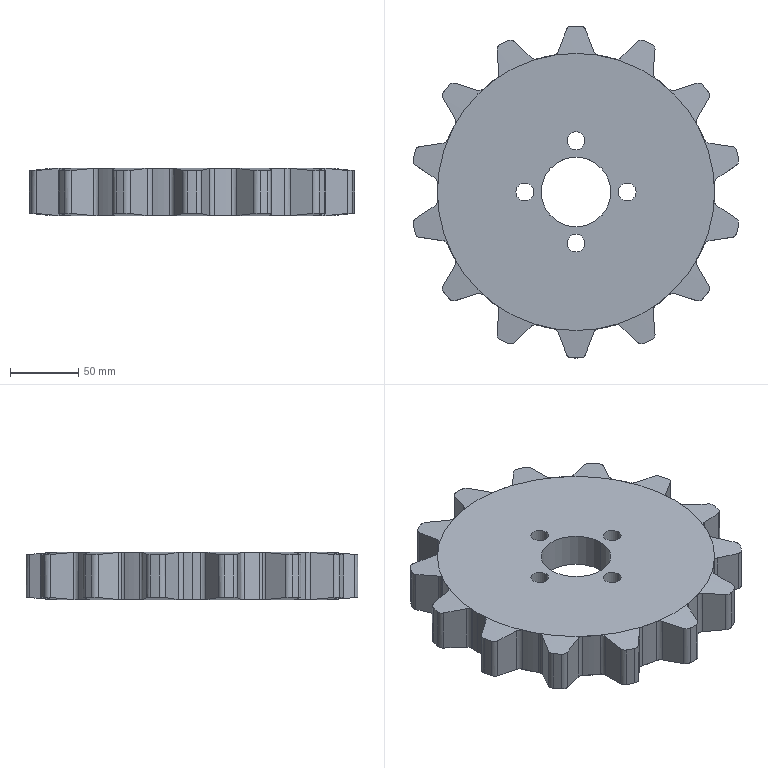Part | SolidWorks | features ICE 4, CirPattern 1, Extrusion 1, RevCut 1 | 1 solid | 172 faces | box 238.389 x 243 x 35 mm | volume 1174087 mm3 | cylinder 109 | plane 59 | cone 4 | commonest cylinder face diameters 8.559 x68 203 x15 243 x14 13 x8 51 x2 101 x2